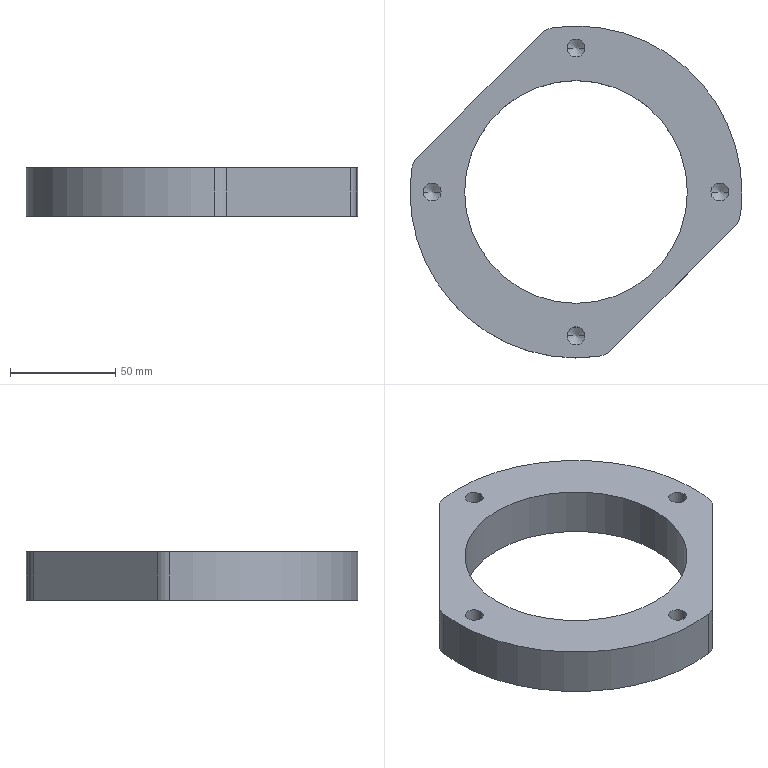Part | SolidWorks | features FlatPattern 1, HoleWzd 1, ICE 1, SMBaseFlange 1, SheetMetal 1 | 1 solid | 29 faces | box 158 x 158 x 23 mm | volume 204311 mm3 | cylinder 17 | cone 8 | plane 4 | commonest cylinder face diameters 8.5 x8 20 x4 158 x3 106 x2
STEP:
#1=CARTESIAN_POINT('',(-4.25,68.5,-18.));
#2=VERTEX_POINT('',#1);
#3=CARTESIAN_POINT('',(4.25,68.5,-18.));
#4=VERTEX_POINT('',#3);
#5=CARTESIAN_POINT('',(0.,68.5,-18.));
#6=DIRECTION('',(0.,0.,1.));
#7=DIRECTION('',(1.,0.,0.));
#8=AXIS2_PLACEMENT_3D('',#5,#6,#7);
#9=CIRCLE('',#8,4.25);
#10=EDGE_CURVE('',#2,#4,#9,.T.);
#11=ORIENTED_EDGE('',*,*,#10,.F.);
#12=CARTESIAN_POINT('',(-4.25,68.5,0.));
#13=VERTEX_POINT('',#12);
#14=CARTESIAN_POINT('',(-4.25,68.5,0.));
#15=DIRECTION('',(0.,0.,1.));
#16=VECTOR('',#15,1000.);
#17=LINE('',#14,#16);
#18=EDGE_CURVE('',#2,#13,#17,.T.);
#19=ORIENTED_EDGE('',*,*,#18,.T.);
#20=CARTESIAN_POINT('',(4.25,68.5,0.));
#21=VERTEX_POINT('',#20);
#22=CARTESIAN_POINT('',(0.,68.5,0.));
#23=DIRECTION('',(0.,0.,1.));
#24=DIRECTION('',(1.,0.,0.));
#25=AXIS2_PLACEMENT_3D('',#22,#23,#24);
#26=CIRCLE('',#25,4.25);
#27=EDGE_CURVE('',#13,#21,#26,.T.);
#28=ORIENTED_EDGE('',*,*,#27,.T.);
#29=CARTESIAN_POINT('',(4.25,68.5,0.));
#30=DIRECTION('',(0.,0.,1.));
#31=VECTOR('',#30,1000.);
#32=LINE('',#29,#31);
#33=EDGE_CURVE('',#4,#21,#32,.T.);
#34=ORIENTED_EDGE('',*,*,#33,.F.);
#35=EDGE_LOOP('',(#11,#19,#28,#34));
#36=FACE_OUTER_BOUND('',#35,.T.);
#37=CARTESIAN_POINT('',(0.,68.5,0.));
#38=DIRECTION('',(0.,0.,1.));
#39=DIRECTION('',(1.,0.,0.));
#40=AXIS2_PLACEMENT_3D('',#37,#38,#39);
#41=CYLINDRICAL_SURFACE('',#40,4.25);
#42=ADVANCED_FACE('',(#36),#41,.F.);
#43=CARTESIAN_POINT('',(0.,68.5,-20.554));
#44=VERTEX_POINT('',#43);
#45=CARTESIAN_POINT('',(4.25,68.5,-18.));
#46=DIRECTION('',(0.8572,0.,0.515));
#47=VECTOR('',#46,1000.);
#48=LINE('',#45,#47);
#49=EDGE_CURVE('',#44,#4,#48,.T.);
#50=ORIENTED_EDGE('',*,*,#49,.F.);
#51=CARTESIAN_POINT('',(-4.25,68.5,-18.));
#52=DIRECTION('',(-0.8572,0.,0.515));
#53=VECTOR('',#52,1000.);
#54=LINE('',#51,#53);
#55=EDGE_CURVE('',#44,#2,#54,.T.);
#56=ORIENTED_EDGE('',*,*,#55,.T.);
#57=ORIENTED_EDGE('',*,*,#10,.T.);
#58=EDGE_LOOP('',(#50,#56,#57));
#59=FACE_OUTER_BOUND('',#58,.T.);
#60=CARTESIAN_POINT('',(0.,68.5,-18.));
#61=DIRECTION('',(0.,0.,1.));
#62=DIRECTION('',(1.,0.,0.));
#63=AXIS2_PLACEMENT_3D('',#60,#61,#62);
#64=CONICAL_SURFACE('',#63,4.25,1.03);
#65=ADVANCED_FACE('',(#59),#64,.F.);
#66=CARTESIAN_POINT('',(64.25,0.,-18.));
#67=VERTEX_POINT('',#66);
#68=CARTESIAN_POINT('',(72.75,0.,-18.));
#69=VERTEX_POINT('',#68);
#70=CARTESIAN_POINT('',(68.5,0.,-18.));
#71=DIRECTION('',(0.,0.,1.));
#72=DIRECTION('',(1.,0.,0.));
#73=AXIS2_PLACEMENT_3D('',#70,#71,#72);
#74=CIRCLE('',#73,4.25);
#75=EDGE_CURVE('',#67,#69,#74,.T.);
#76=ORIENTED_EDGE('',*,*,#75,.F.);
#77=CARTESIAN_POINT('',(64.25,0.,0.));
#78=VERTEX_POINT('',#77);
#79=CARTESIAN_POINT('',(64.25,0.,0.));
#80=DIRECTION('',(0.,0.,1.));
#81=VECTOR('',#80,1000.);
#82=LINE('',#79,#81);
#83=EDGE_CURVE('',#67,#78,#82,.T.);
#84=ORIENTED_EDGE('',*,*,#83,.T.);
#85=CARTESIAN_POINT('',(72.75,0.,0.));
#86=VERTEX_POINT('',#85);
#87=CARTESIAN_POINT('',(68.5,0.,0.));
#88=DIRECTION('',(0.,0.,1.));
#89=DIRECTION('',(1.,0.,0.));
#90=AXIS2_PLACEMENT_3D('',#87,#88,#89);
#91=CIRCLE('',#90,4.25);
#92=EDGE_CURVE('',#78,#86,#91,.T.);
#93=ORIENTED_EDGE('',*,*,#92,.T.);
#94=CARTESIAN_POINT('',(72.75,0.,0.));
#95=DIRECTION('',(0.,0.,1.));
#96=VECTOR('',#95,1000.);
#97=LINE('',#94,#96);
#98=EDGE_CURVE('',#69,#86,#97,.T.);
#99=ORIENTED_EDGE('',*,*,#98,.F.);
#100=EDGE_LOOP('',(#76,#84,#93,#99));
#101=FACE_OUTER_BOUND('',#100,.T.);
#102=CARTESIAN_POINT('',(68.5,0.,0.));
#103=DIRECTION('',(0.,0.,1.));
#104=DIRECTION('',(1.,0.,0.));
#105=AXIS2_PLACEMENT_3D('',#102,#103,#104);
#106=CYLINDRICAL_SURFACE('',#105,4.25);
#107=ADVANCED_FACE('',(#101),#106,.F.);
#108=CARTESIAN_POINT('',(68.5,0.,-20.554));
#109=VERTEX_POINT('',#108);
#110=CARTESIAN_POINT('',(72.75,0.,-18.));
#111=DIRECTION('',(0.8572,0.,0.515));
#112=VECTOR('',#111,1000.);
#113=LINE('',#110,#112);
#114=EDGE_CURVE('',#109,#69,#113,.T.);
#115=ORIENTED_EDGE('',*,*,#114,.F.);
#116=CARTESIAN_POINT('',(64.25,0.,-18.));
#117=DIRECTION('',(-0.8572,0.,0.515));
#118=VECTOR('',#117,1000.);
#119=LINE('',#116,#118);
#120=EDGE_CURVE('',#109,#67,#119,.T.);
#121=ORIENTED_EDGE('',*,*,#120,.T.);
#122=ORIENTED_EDGE('',*,*,#75,.T.);
#123=EDGE_LOOP('',(#115,#121,#122));
#124=FACE_OUTER_BOUND('',#123,.T.);
#125=CARTESIAN_POINT('',(68.5,0.,-18.));
#126=DIRECTION('',(0.,0.,1.));
#127=DIRECTION('',(1.,0.,0.));
#128=AXIS2_PLACEMENT_3D('',#125,#126,#127);
#129=CONICAL_SURFACE('',#128,4.25,1.03);
#130=ADVANCED_FACE('',(#124),#129,.F.);
#131=CARTESIAN_POINT('',(-4.25,-68.5,-18.));
#132=VERTEX_POINT('',#131);
#133=CARTESIAN_POINT('',(4.25,-68.5,-18.));
#134=VERTEX_POINT('',#133);
#135=CARTESIAN_POINT('',(0.,-68.5,-18.));
#136=DIRECTION('',(0.,0.,1.));
#137=DIRECTION('',(1.,0.,0.));
#138=AXIS2_PLACEMENT_3D('',#135,#136,#137);
#139=CIRCLE('',#138,4.25);
#140=EDGE_CURVE('',#132,#134,#139,.T.);
#141=ORIENTED_EDGE('',*,*,#140,.F.);
#142=CARTESIAN_POINT('',(-4.25,-68.5,0.));
#143=VERTEX_POINT('',#142);
#144=CARTESIAN_POINT('',(-4.25,-68.5,0.));
#145=DIRECTION('',(0.,0.,1.));
#146=VECTOR('',#145,1000.);
#147=LINE('',#144,#146);
#148=EDGE_CURVE('',#132,#143,#147,.T.);
#149=ORIENTED_EDGE('',*,*,#148,.T.);
#150=CARTESIAN_POINT('',(4.25,-68.5,0.));
#151=VERTEX_POINT('',#150);
#152=CARTESIAN_POINT('',(0.,-68.5,0.));
#153=DIRECTION('',(0.,0.,1.));
#154=DIRECTION('',(1.,0.,0.));
#155=AXIS2_PLACEMENT_3D('',#152,#153,#154);
#156=CIRCLE('',#155,4.25);
#157=EDGE_CURVE('',#143,#151,#156,.T.);
#158=ORIENTED_EDGE('',*,*,#157,.T.);
#159=CARTESIAN_POINT('',(4.25,-68.5,0.));
#160=DIRECTION('',(0.,0.,1.));
#161=VECTOR('',#160,1000.);
#162=LINE('',#159,#161);
#163=EDGE_CURVE('',#134,#151,#162,.T.);
#164=ORIENTED_EDGE('',*,*,#163,.F.);
#165=EDGE_LOOP('',(#141,#149,#158,#164));
#166=FACE_OUTER_BOUND('',#165,.T.);
#167=CARTESIAN_POINT('',(0.,-68.5,0.));
#168=DIRECTION('',(0.,0.,1.));
#169=DIRECTION('',(1.,0.,0.));
#170=AXIS2_PLACEMENT_3D('',#167,#168,#169);
#171=CYLINDRICAL_SURFACE('',#170,4.25);
#172=ADVANCED_FACE('',(#166),#171,.F.);
#173=CARTESIAN_POINT('',(0.,-68.5,-20.554));
#174=VERTEX_POINT('',#173);
#175=CARTESIAN_POINT('',(4.25,-68.5,-18.));
#176=DIRECTION('',(0.8572,0.,0.515));
#177=VECTOR('',#176,1000.);
#178=LINE('',#175,#177);
#179=EDGE_CURVE('',#174,#134,#178,.T.);
#180=ORIENTED_EDGE('',*,*,#179,.F.);
#181=CARTESIAN_POINT('',(-4.25,-68.5,-18.));
#182=DIRECTION('',(-0.8572,0.,0.515));
#183=VECTOR('',#182,1000.);
#184=LINE('',#181,#183);
#185=EDGE_CURVE('',#174,#132,#184,.T.);
#186=ORIENTED_EDGE('',*,*,#185,.T.);
#187=ORIENTED_EDGE('',*,*,#140,.T.);
#188=EDGE_LOOP('',(#180,#186,#187));
#189=FACE_OUTER_BOUND('',#188,.T.);
#190=CARTESIAN_POINT('',(0.,-68.5,-18.));
#191=DIRECTION('',(0.,0.,1.));
#192=DIRECTION('',(1.,0.,0.));
#193=AXIS2_PLACEMENT_3D('',#190,#191,#192);
#194=CONICAL_SURFACE('',#193,4.25,1.03);
#195=ADVANCED_FACE('',(#189),#194,.F.);
#196=CARTESIAN_POINT('',(-72.75,0.,-18.));
#197=VERTEX_POINT('',#196);
#198=CARTESIAN_POINT('',(-64.25,0.,-18.));
#199=VERTEX_POINT('',#198);
#200=CARTESIAN_POINT('',(-68.5,0.,-18.));
#201=DIRECTION('',(0.,0.,1.));
#202=DIRECTION('',(1.,0.,0.));
#203=AXIS2_PLACEMENT_3D('',#200,#201,#202);
#204=CIRCLE('',#203,4.25);
#205=EDGE_CURVE('',#197,#199,#204,.T.);
#206=ORIENTED_EDGE('',*,*,#205,.F.);
#207=CARTESIAN_POINT('',(-72.75,0.,0.));
#208=VERTEX_POINT('',#207);
#209=CARTESIAN_POINT('',(-72.75,0.,0.));
#210=DIRECTION('',(0.,0.,1.));
#211=VECTOR('',#210,1000.);
#212=LINE('',#209,#211);
#213=EDGE_CURVE('',#197,#208,#212,.T.);
#214=ORIENTED_EDGE('',*,*,#213,.T.);
#215=CARTESIAN_POINT('',(-64.25,0.,0.));
#216=VERTEX_POINT('',#215);
#217=CARTESIAN_POINT('',(-68.5,0.,0.));
#218=DIRECTION('',(0.,0.,1.));
#219=DIRECTION('',(1.,0.,0.));
#220=AXIS2_PLACEMENT_3D('',#217,#218,#219);
#221=CIRCLE('',#220,4.25);
#222=EDGE_CURVE('',#208,#216,#221,.T.);
#223=ORIENTED_EDGE('',*,*,#222,.T.);
#224=CARTESIAN_POINT('',(-64.25,0.,0.));
#225=DIRECTION('',(0.,0.,1.));
#226=VECTOR('',#225,1000.);
#227=LINE('',#224,#226);
#228=EDGE_CURVE('',#199,#216,#227,.T.);
#229=ORIENTED_EDGE('',*,*,#228,.F.);
#230=EDGE_LOOP('',(#206,#214,#223,#229));
#231=FACE_OUTER_BOUND('',#230,.T.);
#232=CARTESIAN_POINT('',(-68.5,0.,0.));
#233=DIRECTION('',(0.,0.,1.));
#234=DIRECTION('',(1.,0.,0.));
#235=AXIS2_PLACEMENT_3D('',#232,#233,#234);
#236=CYLINDRICAL_SURFACE('',#235,4.25);
#237=ADVANCED_FACE('',(#231),#236,.F.);
#238=CARTESIAN_POINT('',(-68.5,0.,-20.554));
#239=VERTEX_POINT('',#238);
#240=CARTESIAN_POINT('',(-64.25,0.,-18.));
#241=DIRECTION('',(0.8572,0.,0.515));
#242=VECTOR('',#241,1000.);
#243=LINE('',#240,#242);
#244=EDGE_CURVE('',#239,#199,#243,.T.);
#245=ORIENTED_EDGE('',*,*,#244,.F.);
#246=CARTESIAN_POINT('',(-72.75,0.,-18.));
#247=DIRECTION('',(-0.8572,0.,0.515));
#248=VECTOR('',#247,1000.);
#249=LINE('',#246,#248);
#250=EDGE_CURVE('',#239,#197,#249,.T.);
#251=ORIENTED_EDGE('',*,*,#250,.T.);
#252=ORIENTED_EDGE('',*,*,#205,.T.);
#253=EDGE_LOOP('',(#245,#251,#252));
#254=FACE_OUTER_BOUND('',#253,.T.);
#255=CARTESIAN_POINT('',(-68.5,0.,-18.));
#256=DIRECTION('',(0.,0.,1.));
#257=DIRECTION('',(1.,0.,0.));
#258=AXIS2_PLACEMENT_3D('',#255,#256,#257);
#259=CONICAL_SURFACE('',#258,4.25,1.03);
#260=ADVANCED_FACE('',(#254),#259,.F.);
#261=CARTESIAN_POINT('',(-53.,0.,-23.));
#262=VERTEX_POINT('',#261);
#263=CARTESIAN_POINT('',(53.,0.,-23.));
#264=VERTEX_POINT('',#263);
#265=CARTESIAN_POINT('',(0.,0.,-23.));
#266=DIRECTION('',(0.,0.,1.));
#267=DIRECTION('',(1.,0.,0.));
#268=AXIS2_PLACEMENT_3D('',#265,#266,#267);
#269=CIRCLE('',#268,53.);
#270=EDGE_CURVE('',#262,#264,#269,.T.);
#271=ORIENTED_EDGE('',*,*,#270,.F.);
#272=CARTESIAN_POINT('',(-53.,0.,0.));
#273=VERTEX_POINT('',#272);
#274=CARTESIAN_POINT('',(-53.,0.,-23.));
#275=DIRECTION('',(0.,0.,1.));
#276=VECTOR('',#275,1000.);
#277=LINE('',#274,#276);
#278=EDGE_CURVE('',#262,#273,#277,.T.);
#279=ORIENTED_EDGE('',*,*,#278,.T.);
#280=CARTESIAN_POINT('',(53.,0.,0.));
#281=VERTEX_POINT('',#280);
#282=CARTESIAN_POINT('',(0.,0.,0.));
#283=DIRECTION('',(0.,0.,1.));
#284=DIRECTION('',(1.,0.,0.));
#285=AXIS2_PLACEMENT_3D('',#282,#283,#284);
#286=CIRCLE('',#285,53.);
#287=EDGE_CURVE('',#273,#281,#286,.T.);
#288=ORIENTED_EDGE('',*,*,#287,.T.);
#289=CARTESIAN_POINT('',(53.,0.,-23.));
#290=DIRECTION('',(0.,0.,1.));
#291=VECTOR('',#290,1000.);
#292=LINE('',#289,#291);
#293=EDGE_CURVE('',#264,#281,#292,.T.);
#294=ORIENTED_EDGE('',*,*,#293,.F.);
#295=EDGE_LOOP('',(#271,#279,#288,#294));
#296=FACE_OUTER_BOUND('',#295,.T.);
#297=CARTESIAN_POINT('',(0.,0.,-23.));
#298=DIRECTION('',(0.,0.,1.));
#299=DIRECTION('',(1.,0.,0.));
#300=AXIS2_PLACEMENT_3D('',#297,#298,#299);
#301=CYLINDRICAL_SURFACE('',#300,53.);
#302=ADVANCED_FACE('',(#296),#301,.F.);
#303=CARTESIAN_POINT('',(78.259,-10.796,-23.));
#304=VERTEX_POINT('',#303);
#305=CARTESIAN_POINT('',(79.,0.,-23.));
#306=VERTEX_POINT('',#305);
#307=CARTESIAN_POINT('',(0.,0.,-23.));
#308=DIRECTION('',(0.,0.,1.));
#309=DIRECTION('',(1.,0.,0.));
#310=AXIS2_PLACEMENT_3D('',#307,#308,#309);
#311=CIRCLE('',#310,79.);
#312=EDGE_CURVE('',#304,#306,#311,.T.);
#313=ORIENTED_EDGE('',*,*,#312,.T.);
#314=CARTESIAN_POINT('',(79.,0.,0.));
#315=VERTEX_POINT('',#314);
#316=CARTESIAN_POINT('',(79.,0.,-23.));
#317=DIRECTION('',(0.,0.,1.));
#318=VECTOR('',#317,1000.);
#319=LINE('',#316,#318);
#320=EDGE_CURVE('',#306,#315,#319,.T.);
#321=ORIENTED_EDGE('',*,*,#320,.T.);
#322=CARTESIAN_POINT('',(78.259,-10.796,0.));
#323=VERTEX_POINT('',#322);
#324=CARTESIAN_POINT('',(0.,0.,0.));
#325=DIRECTION('',(0.,0.,1.));
#326=DIRECTION('',(1.,0.,0.));
#327=AXIS2_PLACEMENT_3D('',#324,#325,#326);
#328=CIRCLE('',#327,79.);
#329=EDGE_CURVE('',#323,#315,#328,.T.);
#330=ORIENTED_EDGE('',*,*,#329,.F.);
#331=CARTESIAN_POINT('',(78.259,-10.796,-23.));
#332=DIRECTION('',(0.,0.,1.));
#333=VECTOR('',#332,1000.);
#334=LINE('',#331,#333);
#335=EDGE_CURVE('',#304,#323,#334,.T.);
#336=ORIENTED_EDGE('',*,*,#335,.F.);
#337=EDGE_LOOP('',(#313,#321,#330,#336));
#338=FACE_OUTER_BOUND('',#337,.T.);
#339=CARTESIAN_POINT('',(0.,0.,-23.));
#340=DIRECTION('',(0.,0.,1.));
#341=DIRECTION('',(1.,0.,0.));
#342=AXIS2_PLACEMENT_3D('',#339,#340,#341);
#343=CYLINDRICAL_SURFACE('',#342,79.);
#344=ADVANCED_FACE('',(#338),#343,.T.);
#345=CARTESIAN_POINT('',(75.424,-16.5,0.));
#346=VERTEX_POINT('',#345);
#347=CARTESIAN_POINT('',(68.353,-9.429,0.));
#348=DIRECTION('',(0.,0.,1.));
#349=DIRECTION('',(1.,0.,0.));
#350=AXIS2_PLACEMENT_3D('',#347,#348,#349);
#351=CIRCLE('',#350,10.);
#352=EDGE_CURVE('',#346,#323,#351,.T.);
#353=ORIENTED_EDGE('',*,*,#352,.F.);
#354=CARTESIAN_POINT('',(75.424,-16.5,-23.));
#355=VERTEX_POINT('',#354);
#356=CARTESIAN_POINT('',(75.424,-16.5,-23.));
#357=DIRECTION('',(0.,0.,1.));
#358=VECTOR('',#357,1000.);
#359=LINE('',#356,#358);
#360=EDGE_CURVE('',#355,#346,#359,.T.);
#361=ORIENTED_EDGE('',*,*,#360,.F.);
#362=CARTESIAN_POINT('',(68.353,-9.429,-23.));
#363=DIRECTION('',(0.,0.,1.));
#364=DIRECTION('',(1.,0.,0.));
#365=AXIS2_PLACEMENT_3D('',#362,#363,#364);
#366=CIRCLE('',#365,10.);
#367=EDGE_CURVE('',#355,#304,#366,.T.);
#368=ORIENTED_EDGE('',*,*,#367,.T.);
#369=ORIENTED_EDGE('',*,*,#335,.T.);
#370=EDGE_LOOP('',(#353,#361,#368,#369));
#371=FACE_OUTER_BOUND('',#370,.T.);
#372=CARTESIAN_POINT('',(68.353,-9.429,-23.));
#373=DIRECTION('',(0.,0.,1.));
#374=DIRECTION('',(1.,0.,0.));
#375=AXIS2_PLACEMENT_3D('',#372,#373,#374);
#376=CYLINDRICAL_SURFACE('',#375,10.);
#377=ADVANCED_FACE('',(#371),#376,.T.);
#378=CARTESIAN_POINT('',(16.5,-75.424,0.));
#379=VERTEX_POINT('',#378);
#380=CARTESIAN_POINT('',(16.5,-75.424,0.));
#381=DIRECTION('',(0.7071,0.7071,0.));
#382=VECTOR('',#381,1000.);
#383=LINE('',#380,#382);
#384=EDGE_CURVE('',#379,#346,#383,.T.);
#385=ORIENTED_EDGE('',*,*,#384,.F.);
#386=CARTESIAN_POINT('',(16.5,-75.424,-23.));
#387=VERTEX_POINT('',#386);
#388=CARTESIAN_POINT('',(16.5,-75.424,-23.));
#389=DIRECTION('',(0.,0.,1.));
#390=VECTOR('',#389,1000.);
#391=LINE('',#388,#390);
#392=EDGE_CURVE('',#387,#379,#391,.T.);
#393=ORIENTED_EDGE('',*,*,#392,.F.);
#394=CARTESIAN_POINT('',(16.5,-75.424,-23.));
#395=DIRECTION('',(0.7071,0.7071,0.));
#396=VECTOR('',#395,1000.);
#397=LINE('',#394,#396);
#398=EDGE_CURVE('',#387,#355,#397,.T.);
#399=ORIENTED_EDGE('',*,*,#398,.T.);
#400=ORIENTED_EDGE('',*,*,#360,.T.);
#401=EDGE_LOOP('',(#385,#393,#399,#400));
#402=FACE_OUTER_BOUND('',#401,.T.);
#403=CARTESIAN_POINT('',(16.5,-75.424,-23.));
#404=DIRECTION('',(0.7071,-0.7071,0.));
#405=DIRECTION('',(0.7071,0.7071,0.));
#406=AXIS2_PLACEMENT_3D('',#403,#404,#405);
#407=PLANE('',#406);
#408=ADVANCED_FACE('',(#402),#407,.T.);
#409=CARTESIAN_POINT('',(10.796,-78.259,0.));
#410=VERTEX_POINT('',#409);
#411=CARTESIAN_POINT('',(9.429,-68.353,0.));
#412=DIRECTION('',(0.,0.,1.));
#413=DIRECTION('',(-1.,0.,0.));
#414=AXIS2_PLACEMENT_3D('',#411,#412,#413);
#415=CIRCLE('',#414,10.);
#416=EDGE_CURVE('',#410,#379,#415,.T.);
#417=ORIENTED_EDGE('',*,*,#416,.F.);
#418=CARTESIAN_POINT('',(10.796,-78.259,-23.));
#419=VERTEX_POINT('',#418);
#420=CARTESIAN_POINT('',(10.796,-78.259,-23.));
#421=DIRECTION('',(0.,0.,1.));
#422=VECTOR('',#421,1000.);
#423=LINE('',#420,#422);
#424=EDGE_CURVE('',#419,#410,#423,.T.);
#425=ORIENTED_EDGE('',*,*,#424,.F.);
#426=CARTESIAN_POINT('',(9.429,-68.353,-23.));
#427=DIRECTION('',(0.,0.,1.));
#428=DIRECTION('',(-1.,0.,0.));
#429=AXIS2_PLACEMENT_3D('',#426,#427,#428);
#430=CIRCLE('',#429,10.);
#431=EDGE_CURVE('',#419,#387,#430,.T.);
#432=ORIENTED_EDGE('',*,*,#431,.T.);
#433=ORIENTED_EDGE('',*,*,#392,.T.);
#434=EDGE_LOOP('',(#417,#425,#432,#433));
#435=FACE_OUTER_BOUND('',#434,.T.);
#436=CARTESIAN_POINT('',(9.429,-68.353,-23.));
#437=DIRECTION('',(0.,0.,1.));
#438=DIRECTION('',(1.,0.,0.));
#439=AXIS2_PLACEMENT_3D('',#436,#437,#438);
#440=CYLINDRICAL_SURFACE('',#439,10.);
#441=ADVANCED_FACE('',(#435),#440,.T.);
#442=CARTESIAN_POINT('',(-78.259,10.796,0.));
#443=VERTEX_POINT('',#442);
#444=CARTESIAN_POINT('',(0.,0.,0.));
#445=DIRECTION('',(0.,0.,1.));
#446=DIRECTION('',(1.,0.,0.));
#447=AXIS2_PLACEMENT_3D('',#444,#445,#446);
#448=CIRCLE('',#447,79.);
#449=EDGE_CURVE('',#443,#410,#448,.T.);
#450=ORIENTED_EDGE('',*,*,#449,.F.);
#451=CARTESIAN_POINT('',(-78.259,10.796,-23.));
#452=VERTEX_POINT('',#451);
#453=CARTESIAN_POINT('',(-78.259,10.796,-23.));
#454=DIRECTION('',(0.,0.,1.));
#455=VECTOR('',#454,1000.);
#456=LINE('',#453,#455);
#457=EDGE_CURVE('',#452,#443,#456,.T.);
#458=ORIENTED_EDGE('',*,*,#457,.F.);
#459=CARTESIAN_POINT('',(0.,0.,-23.));
#460=DIRECTION('',(0.,0.,1.));
#461=DIRECTION('',(1.,0.,0.));
#462=AXIS2_PLACEMENT_3D('',#459,#460,#461);
#463=CIRCLE('',#462,79.);
#464=EDGE_CURVE('',#452,#419,#463,.T.);
#465=ORIENTED_EDGE('',*,*,#464,.T.);
#466=ORIENTED_EDGE('',*,*,#424,.T.);
#467=EDGE_LOOP('',(#450,#458,#465,#466));
#468=FACE_OUTER_BOUND('',#467,.T.);
#469=CARTESIAN_POINT('',(0.,0.,-23.));
#470=DIRECTION('',(0.,0.,1.));
#471=DIRECTION('',(1.,0.,0.));
#472=AXIS2_PLACEMENT_3D('',#469,#470,#471);
#473=CYLINDRICAL_SURFACE('',#472,79.);
#474=ADVANCED_FACE('',(#468),#473,.T.);
#475=CARTESIAN_POINT('',(-75.424,16.5,0.));
#476=VERTEX_POINT('',#475);
#477=CARTESIAN_POINT('',(-68.353,9.429,0.));
#478=DIRECTION('',(0.,0.,1.));
#479=DIRECTION('',(1.,0.,0.));
#480=AXIS2_PLACEMENT_3D('',#477,#478,#479);
#481=CIRCLE('',#480,10.);
#482=EDGE_CURVE('',#476,#443,#481,.T.);
#483=ORIENTED_EDGE('',*,*,#482,.F.);
#484=CARTESIAN_POINT('',(-75.424,16.5,-23.));
#485=VERTEX_POINT('',#484);
#486=CARTESIAN_POINT('',(-75.424,16.5,-23.));
#487=DIRECTION('',(0.,0.,1.));
#488=VECTOR('',#487,1000.);
#489=LINE('',#486,#488);
#490=EDGE_CURVE('',#485,#476,#489,.T.);
#491=ORIENTED_EDGE('',*,*,#490,.F.);
#492=CARTESIAN_POINT('',(-68.353,9.429,-23.));
#493=DIRECTION('',(0.,0.,1.));
#494=DIRECTION('',(1.,0.,0.));
#495=AXIS2_PLACEMENT_3D('',#492,#493,#494);
#496=CIRCLE('',#495,10.);
#497=EDGE_CURVE('',#485,#452,#496,.T.);
#498=ORIENTED_EDGE('',*,*,#497,.T.);
#499=ORIENTED_EDGE('',*,*,#457,.T.);
#500=EDGE_LOOP('',(#483,#491,#498,#499));
#501=FACE_OUTER_BOUND('',#500,.T.);
#502=CARTESIAN_POINT('',(-68.353,9.429,-23.));
#503=DIRECTION('',(0.,0.,1.));
#504=DIRECTION('',(1.,0.,0.));
#505=AXIS2_PLACEMENT_3D('',#502,#503,#504);
#506=CYLINDRICAL_SURFACE('',#505,10.);
#507=ADVANCED_FACE('',(#501),#506,.T.);
#508=CARTESIAN_POINT('',(-16.5,75.424,0.));
#509=VERTEX_POINT('',#508);
#510=CARTESIAN_POINT('',(-75.424,16.5,0.));
#511=DIRECTION('',(-0.7071,-0.7071,0.));
#512=VECTOR('',#511,1000.);
#513=LINE('',#510,#512);
#514=EDGE_CURVE('',#509,#476,#513,.T.);
#515=ORIENTED_EDGE('',*,*,#514,.F.);
#516=CARTESIAN_POINT('',(-16.5,75.424,-23.));
#517=VERTEX_POINT('',#516);
#518=CARTESIAN_POINT('',(-16.5,75.424,-23.));
#519=DIRECTION('',(0.,0.,1.));
#520=VECTOR('',#519,1000.);
#521=LINE('',#518,#520);
#522=EDGE_CURVE('',#517,#509,#521,.T.);
#523=ORIENTED_EDGE('',*,*,#522,.F.);
#524=CARTESIAN_POINT('',(-75.424,16.5,-23.));
#525=DIRECTION('',(-0.7071,-0.7071,0.));
#526=VECTOR('',#525,1000.);
#527=LINE('',#524,#526);
#528=EDGE_CURVE('',#517,#485,#527,.T.);
#529=ORIENTED_EDGE('',*,*,#528,.T.);
#530=ORIENTED_EDGE('',*,*,#490,.T.);
#531=EDGE_LOOP('',(#515,#523,#529,#530));
#532=FACE_OUTER_BOUND('',#531,.T.);
#533=CARTESIAN_POINT('',(-75.424,16.5,-23.));
#534=DIRECTION('',(-0.7071,0.7071,0.));
#535=DIRECTION('',(-0.7071,-0.7071,0.));
#536=AXIS2_PLACEMENT_3D('',#533,#534,#535);
#537=PLANE('',#536);
#538=ADVANCED_FACE('',(#532),#537,.T.);
#539=CARTESIAN_POINT('',(-10.796,78.259,0.));
#540=VERTEX_POINT('',#539);
#541=CARTESIAN_POINT('',(-9.429,68.353,0.));
#542=DIRECTION('',(0.,0.,1.));
#543=DIRECTION('',(-1.,0.,0.));
#544=AXIS2_PLACEMENT_3D('',#541,#542,#543);
#545=CIRCLE('',#544,10.);
#546=EDGE_CURVE('',#540,#509,#545,.T.);
#547=ORIENTED_EDGE('',*,*,#546,.F.);
#548=CARTESIAN_POINT('',(-10.796,78.259,-23.));
#549=VERTEX_POINT('',#548);
#550=CARTESIAN_POINT('',(-10.796,78.259,-23.));
#551=DIRECTION('',(0.,0.,1.));
#552=VECTOR('',#551,1000.);
#553=LINE('',#550,#552);
#554=EDGE_CURVE('',#549,#540,#553,.T.);
#555=ORIENTED_EDGE('',*,*,#554,.F.);
#556=CARTESIAN_POINT('',(-9.429,68.353,-23.));
#557=DIRECTION('',(0.,0.,1.));
#558=DIRECTION('',(-1.,0.,0.));
#559=AXIS2_PLACEMENT_3D('',#556,#557,#558);
#560=CIRCLE('',#559,10.);
#561=EDGE_CURVE('',#549,#517,#560,.T.);
#562=ORIENTED_EDGE('',*,*,#561,.T.);
#563=ORIENTED_EDGE('',*,*,#522,.T.);
#564=EDGE_LOOP('',(#547,#555,#562,#563));
#565=FACE_OUTER_BOUND('',#564,.T.);
#566=CARTESIAN_POINT('',(-9.429,68.353,-23.));
#567=DIRECTION('',(0.,0.,1.));
#568=DIRECTION('',(1.,0.,0.));
#569=AXIS2_PLACEMENT_3D('',#566,#567,#568);
#570=CYLINDRICAL_SURFACE('',#569,10.);
#571=ADVANCED_FACE('',(#565),#570,.T.);
#572=ORIENTED_EDGE('',*,*,#320,.F.);
#573=CARTESIAN_POINT('',(0.,0.,-23.));
#574=DIRECTION('',(0.,0.,1.));
#575=DIRECTION('',(1.,0.,0.));
#576=AXIS2_PLACEMENT_3D('',#573,#574,#575);
#577=CIRCLE('',#576,79.);
#578=EDGE_CURVE('',#306,#549,#577,.T.);
#579=ORIENTED_EDGE('',*,*,#578,.T.);
#580=ORIENTED_EDGE('',*,*,#554,.T.);
#581=CARTESIAN_POINT('',(0.,0.,0.));
#582=DIRECTION('',(0.,0.,1.));
#583=DIRECTION('',(1.,0.,0.));
#584=AXIS2_PLACEMENT_3D('',#581,#582,#583);
#585=CIRCLE('',#584,79.);
#586=EDGE_CURVE('',#315,#540,#585,.T.);
#587=ORIENTED_EDGE('',*,*,#586,.F.);
#588=EDGE_LOOP('',(#572,#579,#580,#587));
#589=FACE_OUTER_BOUND('',#588,.T.);
#590=CARTESIAN_POINT('',(0.,0.,-23.));
#591=DIRECTION('',(0.,0.,1.));
#592=DIRECTION('',(1.,0.,0.));
#593=AXIS2_PLACEMENT_3D('',#590,#591,#592);
#594=CYLINDRICAL_SURFACE('',#593,79.);
#595=ADVANCED_FACE('',(#589),#594,.T.);
#596=CARTESIAN_POINT('',(0.,0.,-23.));
#597=DIRECTION('',(0.,0.,1.));
#598=DIRECTION('',(1.,0.,0.));
#599=AXIS2_PLACEMENT_3D('',#596,#597,#598);
#600=CIRCLE('',#599,53.);
#601=EDGE_CURVE('',#264,#262,#600,.T.);
#602=ORIENTED_EDGE('',*,*,#601,.T.);
#603=ORIENTED_EDGE('',*,*,#270,.T.);
#604=EDGE_LOOP('',(#602,#603));
#605=FACE_BOUND('',#604,.T.);
#606=ORIENTED_EDGE('',*,*,#367,.F.);
#607=ORIENTED_EDGE('',*,*,#398,.F.);
#608=ORIENTED_EDGE('',*,*,#431,.F.);
#609=ORIENTED_EDGE('',*,*,#464,.F.);
#610=ORIENTED_EDGE('',*,*,#497,.F.);
#611=ORIENTED_EDGE('',*,*,#528,.F.);
#612=ORIENTED_EDGE('',*,*,#561,.F.);
#613=ORIENTED_EDGE('',*,*,#578,.F.);
#614=ORIENTED_EDGE('',*,*,#312,.F.);
#615=EDGE_LOOP('',(#606,#607,#608,#609,#610,#611,#612,#613,#614));
#616=FACE_OUTER_BOUND('',#615,.T.);
#617=CARTESIAN_POINT('',(68.353,-9.429,-23.));
#618=DIRECTION('',(0.,0.,1.));
#619=DIRECTION('',(1.,0.,0.));
#620=AXIS2_PLACEMENT_3D('',#617,#618,#619);
#621=PLANE('',#620);
#622=ADVANCED_FACE('',(#605,#616),#621,.F.);
#623=CARTESIAN_POINT('',(0.,68.5,0.));
#624=DIRECTION('',(0.,0.,1.));
#625=DIRECTION('',(1.,0.,0.));
#626=AXIS2_PLACEMENT_3D('',#623,#624,#625);
#627=CIRCLE('',#626,4.25);
#628=EDGE_CURVE('',#21,#13,#627,.T.);
#629=ORIENTED_EDGE('',*,*,#628,.F.);
#630=ORIENTED_EDGE('',*,*,#27,.F.);
#631=EDGE_LOOP('',(#629,#630));
#632=FACE_BOUND('',#631,.T.);
#633=CARTESIAN_POINT('',(68.5,0.,0.));
#634=DIRECTION('',(0.,0.,1.));
#635=DIRECTION('',(1.,0.,0.));
#636=AXIS2_PLACEMENT_3D('',#633,#634,#635);
#637=CIRCLE('',#636,4.25);
#638=EDGE_CURVE('',#86,#78,#637,.T.);
#639=ORIENTED_EDGE('',*,*,#638,.F.);
#640=ORIENTED_EDGE('',*,*,#92,.F.);
#641=EDGE_LOOP('',(#639,#640));
#642=FACE_BOUND('',#641,.T.);
#643=CARTESIAN_POINT('',(0.,-68.5,0.));
#644=DIRECTION('',(0.,0.,1.));
#645=DIRECTION('',(1.,0.,0.));
#646=AXIS2_PLACEMENT_3D('',#643,#644,#645);
#647=CIRCLE('',#646,4.25);
#648=EDGE_CURVE('',#151,#143,#647,.T.);
#649=ORIENTED_EDGE('',*,*,#648,.F.);
#650=ORIENTED_EDGE('',*,*,#157,.F.);
#651=EDGE_LOOP('',(#649,#650));
#652=FACE_BOUND('',#651,.T.);
#653=CARTESIAN_POINT('',(-68.5,0.,0.));
#654=DIRECTION('',(0.,0.,1.));
#655=DIRECTION('',(1.,0.,0.));
#656=AXIS2_PLACEMENT_3D('',#653,#654,#655);
#657=CIRCLE('',#656,4.25);
#658=EDGE_CURVE('',#216,#208,#657,.T.);
#659=ORIENTED_EDGE('',*,*,#658,.F.);
#660=ORIENTED_EDGE('',*,*,#222,.F.);
#661=EDGE_LOOP('',(#659,#660));
#662=FACE_BOUND('',#661,.T.);
#663=CARTESIAN_POINT('',(0.,0.,0.));
#664=DIRECTION('',(0.,0.,1.));
#665=DIRECTION('',(1.,0.,0.));
#666=AXIS2_PLACEMENT_3D('',#663,#664,#665);
#667=CIRCLE('',#666,53.);
#668=EDGE_CURVE('',#281,#273,#667,.T.);
#669=ORIENTED_EDGE('',*,*,#668,.F.);
#670=ORIENTED_EDGE('',*,*,#287,.F.);
#671=EDGE_LOOP('',(#669,#670));
#672=FACE_BOUND('',#671,.T.);
#673=ORIENTED_EDGE('',*,*,#352,.T.);
#674=ORIENTED_EDGE('',*,*,#329,.T.);
#675=ORIENTED_EDGE('',*,*,#586,.T.);
#676=ORIENTED_EDGE('',*,*,#546,.T.);
#677=ORIENTED_EDGE('',*,*,#514,.T.);
#678=ORIENTED_EDGE('',*,*,#482,.T.);
#679=ORIENTED_EDGE('',*,*,#449,.T.);
#680=ORIENTED_EDGE('',*,*,#416,.T.);
#681=ORIENTED_EDGE('',*,*,#384,.T.);
#682=EDGE_LOOP('',(#673,#674,#675,#676,#677,#678,#679,#680,#681));
#683=FACE_OUTER_BOUND('',#682,.T.);
#684=CARTESIAN_POINT('',(68.353,-9.429,0.));
#685=DIRECTION('',(0.,0.,1.));
#686=DIRECTION('',(1.,0.,0.));
#687=AXIS2_PLACEMENT_3D('',#684,#685,#686);
#688=PLANE('',#687);
#689=ADVANCED_FACE('',(#632,#642,#652,#662,#672,#683),#688,.T.);
#690=ORIENTED_EDGE('',*,*,#278,.F.);
#691=ORIENTED_EDGE('',*,*,#601,.F.);
#692=ORIENTED_EDGE('',*,*,#293,.T.);
#693=ORIENTED_EDGE('',*,*,#668,.T.);
#694=EDGE_LOOP('',(#690,#691,#692,#693));
#695=FACE_OUTER_BOUND('',#694,.T.);
#696=CARTESIAN_POINT('',(0.,0.,-23.));
#697=DIRECTION('',(0.,0.,1.));
#698=DIRECTION('',(1.,0.,0.));
#699=AXIS2_PLACEMENT_3D('',#696,#697,#698);
#700=CYLINDRICAL_SURFACE('',#699,53.);
#701=ADVANCED_FACE('',(#695),#700,.F.);
#702=ORIENTED_EDGE('',*,*,#250,.F.);
#703=ORIENTED_EDGE('',*,*,#244,.T.);
#704=CARTESIAN_POINT('',(-68.5,0.,-18.));
#705=DIRECTION('',(0.,0.,1.));
#706=DIRECTION('',(1.,0.,0.));
#707=AXIS2_PLACEMENT_3D('',#704,#705,#706);
#708=CIRCLE('',#707,4.25);
#709=EDGE_CURVE('',#199,#197,#708,.T.);
#710=ORIENTED_EDGE('',*,*,#709,.T.);
#711=EDGE_LOOP('',(#702,#703,#710));
#712=FACE_OUTER_BOUND('',#711,.T.);
#713=CARTESIAN_POINT('',(-68.5,0.,-18.));
#714=DIRECTION('',(0.,0.,1.));
#715=DIRECTION('',(1.,0.,0.));
#716=AXIS2_PLACEMENT_3D('',#713,#714,#715);
#717=CONICAL_SURFACE('',#716,4.25,1.03);
#718=ADVANCED_FACE('',(#712),#717,.F.);
#719=ORIENTED_EDGE('',*,*,#213,.F.);
#720=ORIENTED_EDGE('',*,*,#709,.F.);
#721=ORIENTED_EDGE('',*,*,#228,.T.);
#722=ORIENTED_EDGE('',*,*,#658,.T.);
#723=EDGE_LOOP('',(#719,#720,#721,#722));
#724=FACE_OUTER_BOUND('',#723,.T.);
#725=CARTESIAN_POINT('',(-68.5,0.,0.));
#726=DIRECTION('',(0.,0.,1.));
#727=DIRECTION('',(1.,0.,0.));
#728=AXIS2_PLACEMENT_3D('',#725,#726,#727);
#729=CYLINDRICAL_SURFACE('',#728,4.25);
#730=ADVANCED_FACE('',(#724),#729,.F.);
#731=ORIENTED_EDGE('',*,*,#185,.F.);
#732=ORIENTED_EDGE('',*,*,#179,.T.);
#733=CARTESIAN_POINT('',(0.,-68.5,-18.));
#734=DIRECTION('',(0.,0.,1.));
#735=DIRECTION('',(1.,0.,0.));
#736=AXIS2_PLACEMENT_3D('',#733,#734,#735);
#737=CIRCLE('',#736,4.25);
#738=EDGE_CURVE('',#134,#132,#737,.T.);
#739=ORIENTED_EDGE('',*,*,#738,.T.);
#740=EDGE_LOOP('',(#731,#732,#739));
#741=FACE_OUTER_BOUND('',#740,.T.);
#742=CARTESIAN_POINT('',(0.,-68.5,-18.));
#743=DIRECTION('',(0.,0.,1.));
#744=DIRECTION('',(1.,0.,0.));
#745=AXIS2_PLACEMENT_3D('',#742,#743,#744);
#746=CONICAL_SURFACE('',#745,4.25,1.03);
#747=ADVANCED_FACE('',(#741),#746,.F.);
#748=ORIENTED_EDGE('',*,*,#148,.F.);
#749=ORIENTED_EDGE('',*,*,#738,.F.);
#750=ORIENTED_EDGE('',*,*,#163,.T.);
#751=ORIENTED_EDGE('',*,*,#648,.T.);
#752=EDGE_LOOP('',(#748,#749,#750,#751));
#753=FACE_OUTER_BOUND('',#752,.T.);
#754=CARTESIAN_POINT('',(0.,-68.5,0.));
#755=DIRECTION('',(0.,0.,1.));
#756=DIRECTION('',(1.,0.,0.));
#757=AXIS2_PLACEMENT_3D('',#754,#755,#756);
#758=CYLINDRICAL_SURFACE('',#757,4.25);
#759=ADVANCED_FACE('',(#753),#758,.F.);
#760=ORIENTED_EDGE('',*,*,#120,.F.);
#761=ORIENTED_EDGE('',*,*,#114,.T.);
#762=CARTESIAN_POINT('',(68.5,0.,-18.));
#763=DIRECTION('',(0.,0.,1.));
#764=DIRECTION('',(1.,0.,0.));
#765=AXIS2_PLACEMENT_3D('',#762,#763,#764);
#766=CIRCLE('',#765,4.25);
#767=EDGE_CURVE('',#69,#67,#766,.T.);
#768=ORIENTED_EDGE('',*,*,#767,.T.);
#769=EDGE_LOOP('',(#760,#761,#768));
#770=FACE_OUTER_BOUND('',#769,.T.);
#771=CARTESIAN_POINT('',(68.5,0.,-18.));
#772=DIRECTION('',(0.,0.,1.));
#773=DIRECTION('',(1.,0.,0.));
#774=AXIS2_PLACEMENT_3D('',#771,#772,#773);
#775=CONICAL_SURFACE('',#774,4.25,1.03);
#776=ADVANCED_FACE('',(#770),#775,.F.);
#777=ORIENTED_EDGE('',*,*,#83,.F.);
#778=ORIENTED_EDGE('',*,*,#767,.F.);
#779=ORIENTED_EDGE('',*,*,#98,.T.);
#780=ORIENTED_EDGE('',*,*,#638,.T.);
#781=EDGE_LOOP('',(#777,#778,#779,#780));
#782=FACE_OUTER_BOUND('',#781,.T.);
#783=CARTESIAN_POINT('',(68.5,0.,0.));
#784=DIRECTION('',(0.,0.,1.));
#785=DIRECTION('',(1.,0.,0.));
#786=AXIS2_PLACEMENT_3D('',#783,#784,#785);
#787=CYLINDRICAL_SURFACE('',#786,4.25);
#788=ADVANCED_FACE('',(#782),#787,.F.);
#789=ORIENTED_EDGE('',*,*,#55,.F.);
#790=ORIENTED_EDGE('',*,*,#49,.T.);
#791=CARTESIAN_POINT('',(0.,68.5,-18.));
#792=DIRECTION('',(0.,0.,1.));
#793=DIRECTION('',(1.,0.,0.));
#794=AXIS2_PLACEMENT_3D('',#791,#792,#793);
#795=CIRCLE('',#794,4.25);
#796=EDGE_CURVE('',#4,#2,#795,.T.);
#797=ORIENTED_EDGE('',*,*,#796,.T.);
#798=EDGE_LOOP('',(#789,#790,#797));
#799=FACE_OUTER_BOUND('',#798,.T.);
#800=CARTESIAN_POINT('',(0.,68.5,-18.));
#801=DIRECTION('',(0.,0.,1.));
#802=DIRECTION('',(1.,0.,0.));
#803=AXIS2_PLACEMENT_3D('',#800,#801,#802);
#804=CONICAL_SURFACE('',#803,4.25,1.03);
#805=ADVANCED_FACE('',(#799),#804,.F.);
#806=ORIENTED_EDGE('',*,*,#18,.F.);
#807=ORIENTED_EDGE('',*,*,#796,.F.);
#808=ORIENTED_EDGE('',*,*,#33,.T.);
#809=ORIENTED_EDGE('',*,*,#628,.T.);
#810=EDGE_LOOP('',(#806,#807,#808,#809));
#811=FACE_OUTER_BOUND('',#810,.T.);
#812=CARTESIAN_POINT('',(0.,68.5,0.));
#813=DIRECTION('',(0.,0.,1.));
#814=DIRECTION('',(1.,0.,0.));
#815=AXIS2_PLACEMENT_3D('',#812,#813,#814);
#816=CYLINDRICAL_SURFACE('',#815,4.25);
#817=ADVANCED_FACE('',(#811),#816,.F.);
#818=CLOSED_SHELL('',(#42,#65,#107,#130,#172,#195,#237,#260,#302,#344,#377,#408,#441,#474,#507,#538,#571,#595,#622,#689,#701,#718,#730,#747,#759,#776,#788,#805,#817));
#819=MANIFOLD_SOLID_BREP('',#818);
#820=CARTESIAN_POINT('',(0.,0.,0.));
#821=DIRECTION('',(0.,0.,1.));
#822=DIRECTION('',(1.,0.,0.));
#823=AXIS2_PLACEMENT_3D('',#820,#821,#822);
#824=(LENGTH_UNIT()NAMED_UNIT(*)SI_UNIT(.MILLI.,.METRE.));
#825=UNCERTAINTY_MEASURE_WITH_UNIT(LENGTH_MEASURE(0.00001),#824,'','');
#826=(NAMED_UNIT(*)PLANE_ANGLE_UNIT()SI_UNIT($,.RADIAN.));
#827=(NAMED_UNIT(*)SI_UNIT($,.STERADIAN.)SOLID_ANGLE_UNIT());
#828=(GEOMETRIC_REPRESENTATION_CONTEXT(3)GLOBAL_UNCERTAINTY_ASSIGNED_CONTEXT((#825))GLOBAL_UNIT_ASSIGNED_CONTEXT((#824,#826,#827))REPRESENTATION_CONTEXT('',''));
#829=ADVANCED_BREP_SHAPE_REPRESENTATION('',(#819,#823),#828);